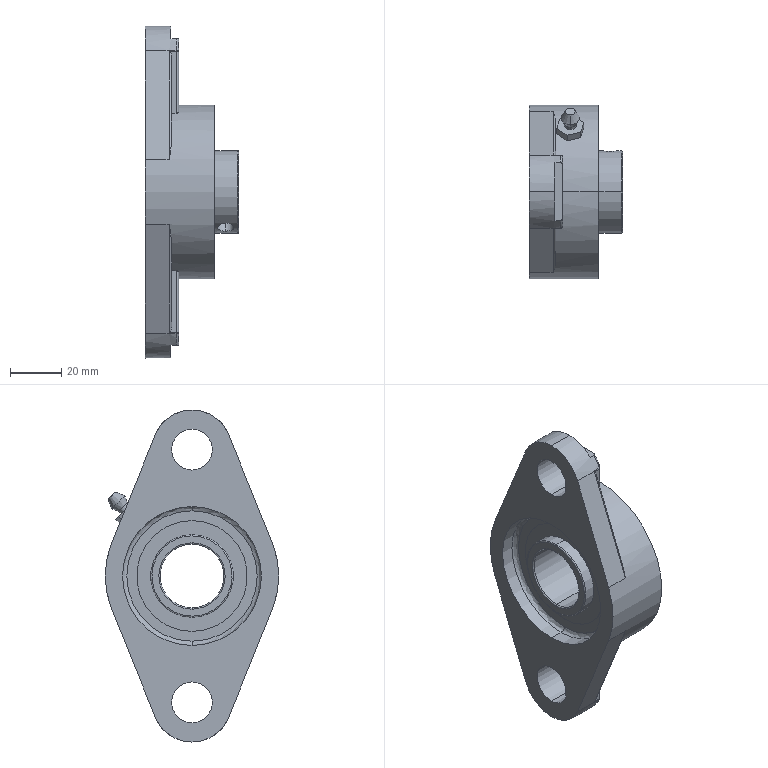Part | SolidWorks | features BaseBody 1, ICE 1 | 1 solid | 105 faces | box 36.46 x 68 x 130 mm | volume 96436 mm3 | cylinder 43 | plane 35 | spline 21 | cone 6 | commonest cylinder face diameters 2 x12 6.25 x4 16 x4 32.35 x4 43.384 x4 51.04 x4